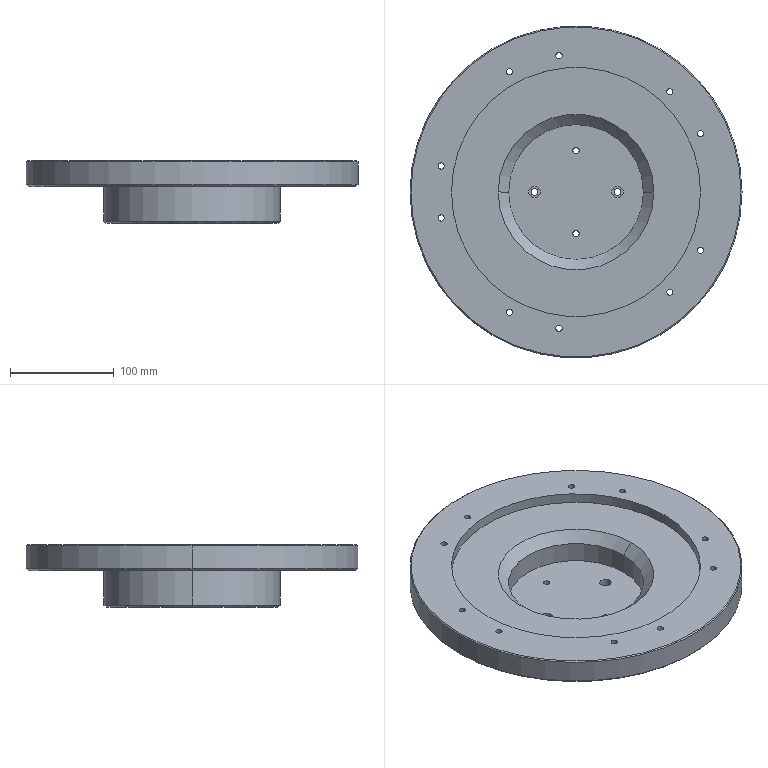CAM job | NX | 3-axis milling, drilling | part box 320 x 320 x 60 mm | stock box 330 x 330 x 65 mm
Tools:
number,name,description,diameter,corner_radius,flute_length,length,flutes
1,D63,Milling Tool-5 Parameters,63.0,0.0,50.0,75.0,2
10,D10,Milling Tool-5 Parameters,10.0,0.0,50.0,75.0,2
20,D20,Milling Tool-5 Parameters,20.0,0.0,50.0,75.0,2
7,D6A45,Milling Tool-5 Parameters,6.0,0.0,3.0,3.0,2
18,5.8ZT,Drilling Tool,5.8,0.0,35.0,50.0,2
19,6.0JD,Milling Tool-5 Parameters,6.0,0.0,30.0,30.0,4
16,6.6ZT,Drilling Tool,6.6,0.0,35.0,50.0,2
6,D6,Milling Tool-5 Parameters,6.0,0.0,50.0,75.0,2
11,D10JING,Milling Tool-5 Parameters,10.0,0.0,50.0,75.0,2
5,D6R0.5,Milling Tool-5 Parameters,6.0,0.5,50.0,75.0,2
Operations:
program,operation,operation_type,tool,method,geometry_group,spindle_rpm,surface_speed,feed_per_tooth,feed_cut,feed_plunge,cut_length_mm,path_length_mm,cut_time_min,machine_time_min
1-330-64_BLANK_AB_GLUE,FLOOR_WALL,VolumeBased25DMillingOperation,D63,METHOD,A,6500.0,1286.0,0.0962,1250.0,100.0,16307.061,17702.413,13.046,13.185
1-330-64_BLANK_AB_GLUE,ZLEVEL_PROFILE,ZLevelMilling,D20,METHOD,A,7000.0,219.0,0.2143,3000.0,1000.0,64232.492,64348.892,21.442,21.454
1-330-64_BLANK_AB_GLUE,ADAPTIVE_MILLING,CavityMilling,D10,METHOD,A,7000.0,219.0,0.2143,3000.0,1000.0,80214.417,81548.669,28.514,28.647
1-330-64_BLANK_AB_GLUE,DRILLING_COPY_1,Operation,D6A45,METHOD,A,3000.0,56.0,0.0333,200.0,0.0,60.0,1318.952,0.3,0.4259
1-330-64_BLANK_AB_GLUE,DRILLING_COPY_1_COPY_COPY_1,Operation,5.8ZT,METHOD,A,2000.0,18.0,0.03,120.0,0.0,364.91,1742.904,3.041,3.179
1-330-64_BLANK_AB_GLUE,DRILLING_COPY_1_COPY_COPY_1_COPY,Operation,6.0JD,METHOD,A,1000.0,9.0,0.01,40.0,0.0,332.0,1677.084,8.3,8.434
1-330-64_BLANK_AB_GLUE,DRILLING_COPY_1_COPY_COPY_1_COPY_1,Operation,6.6ZT,METHOD,A,2000.0,18.0,0.03,120.0,0.0,52.966,328.988,0.4414,0.469
1-330-64_BLANK_AB_GLUE,HOLE_MILLING,CylinderMilling,D6,METHOD,A,7000.0,131.0,0.0714,1000.0,100.0,811.717,1184.318,0.8117,0.849
1-330-64_BLANK_AB_GLUE,ZLEVEL_PROFILE_COPY_COPY_1_COPY_COPY_2_COPY_1,ZLevelMilling,D6R0.5,METHOD,A,7000.0,131.0,0.2143,3000.0,100.0,62738.066,62828.637,20.913,20.922
1-330-64_BLANK_AB_GLUE,FLOOR_WALL_1_COPY_1,VolumeBased25DMillingOperation,D10JING,METHOD,A,7000.0,87.0,0.0714,1000.0,100.0,9236.883,9765.301,9.237,9.299
1-330-64_BLANK_AB_GLUE,ZLEVEL_PROFILE_COPY_1_COPY_COPY_COPY_COPY_2_COPY,ZLevelMilling,D6A45,METHOD,A,7000.0,131.0,0.0714,1000.0,1000.0,1919.848,4412.809,1.92,2.169
1-330-64_BLANK_AB_GLUE,ZLEVEL_PROFILE_COPY_1_COPY_COPY_COPY_COPY_2_COPY_COPY,ZLevelMilling,D6A45,METHOD,A,7000.0,131.0,0.0714,1000.0,1000.0,96.767,865.143,0.0968,0.1736
1-330-64_BLANK_AB_GLUE,CUTTERCOMP11,VolumeBased25DMillingOperation,D10JING,METHOD,A,7000.0,87.0,0.0714,1000.0,100.0,1114.2,1383.289,1.114,1.141
1-330-64_BLANK_AB_GLUE,ZLEVEL_PROFILE_COPY_1,ZLevelMilling,D20,METHOD,A,7000.0,219.0,0.0714,1000.0,1000.0,5534.039,5650.789,5.534,5.546
2-330-64_BLANK_AB_GLUE,FLOOR_WALL_COPY,VolumeBased25DMillingOperation,D63,METHOD,B,6500.0,1286.0,0.0962,1250.0,100.0,3979.818,4033.818,3.184,3.189
2-330-64_BLANK_AB_GLUE,ADAPTIVE_MILLING_COPY,CavityMilling,D10,METHOD,B,7000.0,219.0,0.2143,3000.0,1000.0,145028.394,145396.533,48.349,48.386
2-330-64_BLANK_AB_GLUE,FLOOR_WALL_1_COPY_1_COPY,VolumeBased25DMillingOperation,D10JING,METHOD,B,7000.0,87.0,0.0714,1000.0,100.0,12872.862,13390.857,12.873,12.93
2-330-64_BLANK_AB_GLUE,ZLEVEL_PROFILE_COPY_1_COPY_COPY_COPY_COPY_2_COPY_COPY_1,ZLevelMilling,D6A45,METHOD,B,7000.0,131.0,0.0571,800.0,1000.0,540.533,605.533,0.6753,0.6818
2-330-64_BLANK_AB_GLUE,ZLEVEL_PROFILE_COPY_1_COPY_COPY_COPY_COPY_2_COPY_COPY_1_COPY,ZLevelMilling,D6A45,METHOD,B,7000.0,131.0,0.0571,800.0,1000.0,1011.779,1146.779,1.264,1.278
2-330-64_BLANK_AB_GLUE,CUTTERCOMP11_COPY,VolumeBased25DMillingOperation,D10JING,METHOD,B,7000.0,87.0,0.0714,1000.0,100.0,1146.757,1314.699,1.147,1.164